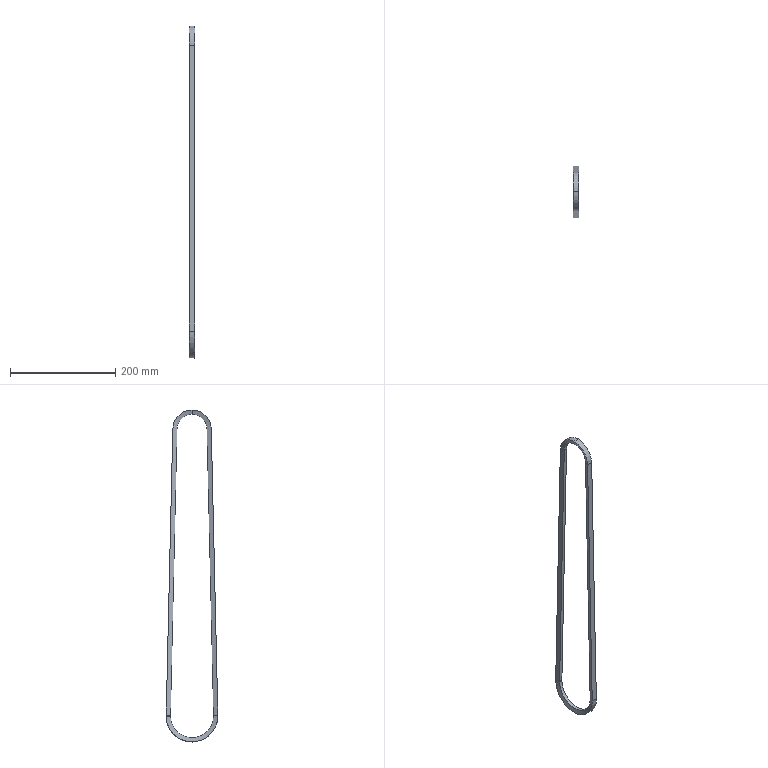Part | STEP file | Long V-belt | 1 solid | 24 faces | box 11 x 98 x 629.5 mm | volume 91301 mm3 | cone 8 | cylinder 8 | plane 8 | commonest cylinder face diameters 57 x2 73 x2 82 x2 98 x2
STEP:
#1=CARTESIAN_POINT('',(3.054,41.,0.));
#2=VERTEX_POINT('',#1);
#3=CARTESIAN_POINT('',(3.054,0.,-41.));
#4=VERTEX_POINT('',#3);
#5=CARTESIAN_POINT('',(3.054,0.,0.));
#6=DIRECTION('',(-1.,0.,0.));
#7=DIRECTION('',(0.,1.,0.));
#8=AXIS2_PLACEMENT_3D('',#5,#6,#7);
#9=CIRCLE('',#8,41.);
#10=EDGE_CURVE('',#2,#4,#9,.T.);
#11=ORIENTED_EDGE('',*,*,#10,.T.);
#12=CARTESIAN_POINT('',(5.5,0.,-49.));
#13=VERTEX_POINT('',#12);
#14=CARTESIAN_POINT('',(3.054,0.,-41.));
#15=DIRECTION('',(0.2924,0.,-0.9563));
#16=VECTOR('',#15,1000.);
#17=LINE('',#14,#16);
#18=EDGE_CURVE('',#4,#13,#17,.T.);
#19=ORIENTED_EDGE('',*,*,#18,.T.);
#20=CARTESIAN_POINT('',(5.5,49.,0.));
#21=VERTEX_POINT('',#20);
#22=CARTESIAN_POINT('',(5.5,0.,0.));
#23=DIRECTION('',(-1.,0.,0.));
#24=DIRECTION('',(0.,1.,0.));
#25=AXIS2_PLACEMENT_3D('',#22,#23,#24);
#26=CIRCLE('',#25,49.);
#27=EDGE_CURVE('',#21,#13,#26,.T.);
#28=ORIENTED_EDGE('',*,*,#27,.F.);
#29=CARTESIAN_POINT('',(3.054,41.,0.));
#30=DIRECTION('',(0.2924,0.9563,0.));
#31=VECTOR('',#30,1000.);
#32=LINE('',#29,#31);
#33=EDGE_CURVE('',#2,#21,#32,.T.);
#34=ORIENTED_EDGE('',*,*,#33,.F.);
#35=EDGE_LOOP('',(#11,#19,#28,#34));
#36=FACE_OUTER_BOUND('',#35,.T.);
#37=CARTESIAN_POINT('',(3.054,0.,0.));
#38=DIRECTION('',(1.,0.,0.));
#39=DIRECTION('',(0.,0.,-1.));
#40=AXIS2_PLACEMENT_3D('',#37,#38,#39);
#41=CONICAL_SURFACE('',#40,41.,1.274);
#42=ADVANCED_FACE('',(#36),#41,.F.);
#43=CARTESIAN_POINT('',(5.5,-36.5,544.098));
#44=VERTEX_POINT('',#43);
#45=CARTESIAN_POINT('',(5.5,0.,580.5));
#46=VERTEX_POINT('',#45);
#47=CARTESIAN_POINT('',(5.5,0.,544.));
#48=DIRECTION('',(-1.,0.,0.));
#49=DIRECTION('',(0.,-1.,0.));
#50=AXIS2_PLACEMENT_3D('',#47,#48,#49);
#51=CIRCLE('',#50,36.5);
#52=EDGE_CURVE('',#44,#46,#51,.T.);
#53=ORIENTED_EDGE('',*,*,#52,.T.);
#54=CARTESIAN_POINT('',(-5.5,0.,580.5));
#55=VERTEX_POINT('',#54);
#56=CARTESIAN_POINT('',(0.,0.,580.5));
#57=DIRECTION('',(-1.,0.,0.));
#58=VECTOR('',#57,1000.);
#59=LINE('',#56,#58);
#60=EDGE_CURVE('',#46,#55,#59,.T.);
#61=ORIENTED_EDGE('',*,*,#60,.T.);
#62=CARTESIAN_POINT('',(-5.5,-36.5,544.098));
#63=VERTEX_POINT('',#62);
#64=CARTESIAN_POINT('',(-5.5,0.,544.));
#65=DIRECTION('',(-1.,0.,0.));
#66=DIRECTION('',(0.,-1.,0.));
#67=AXIS2_PLACEMENT_3D('',#64,#65,#66);
#68=CIRCLE('',#67,36.5);
#69=EDGE_CURVE('',#63,#55,#68,.T.);
#70=ORIENTED_EDGE('',*,*,#69,.F.);
#71=CARTESIAN_POINT('',(0.,-36.5,544.098));
#72=DIRECTION('',(1.,0.,0.));
#73=VECTOR('',#72,1000.);
#74=LINE('',#71,#73);
#75=EDGE_CURVE('',#63,#44,#74,.T.);
#76=ORIENTED_EDGE('',*,*,#75,.T.);
#77=EDGE_LOOP('',(#53,#61,#70,#76));
#78=FACE_OUTER_BOUND('',#77,.T.);
#79=CARTESIAN_POINT('',(0.,0.,544.));
#80=DIRECTION('',(-1.,0.,0.));
#81=DIRECTION('',(0.,0.,1.));
#82=AXIS2_PLACEMENT_3D('',#79,#80,#81);
#83=CYLINDRICAL_SURFACE('',#82,36.5);
#84=ADVANCED_FACE('',(#78),#83,.T.);
#85=CARTESIAN_POINT('',(3.054,0.,572.5));
#86=VERTEX_POINT('',#85);
#87=CARTESIAN_POINT('',(3.054,28.5,544.));
#88=VERTEX_POINT('',#87);
#89=CARTESIAN_POINT('',(3.054,0.,544.));
#90=DIRECTION('',(-1.,0.,0.));
#91=DIRECTION('',(0.,-1.,0.));
#92=AXIS2_PLACEMENT_3D('',#89,#90,#91);
#93=CIRCLE('',#92,28.5);
#94=EDGE_CURVE('',#86,#88,#93,.T.);
#95=ORIENTED_EDGE('',*,*,#94,.F.);
#96=CARTESIAN_POINT('',(-3.054,0.,572.5));
#97=VERTEX_POINT('',#96);
#98=CARTESIAN_POINT('',(0.,0.,572.5));
#99=DIRECTION('',(-1.,0.,0.));
#100=VECTOR('',#99,1000.);
#101=LINE('',#98,#100);
#102=EDGE_CURVE('',#86,#97,#101,.T.);
#103=ORIENTED_EDGE('',*,*,#102,.T.);
#104=CARTESIAN_POINT('',(-3.054,28.5,544.));
#105=VERTEX_POINT('',#104);
#106=CARTESIAN_POINT('',(-3.054,0.,544.));
#107=DIRECTION('',(-1.,0.,0.));
#108=DIRECTION('',(0.,-1.,0.));
#109=AXIS2_PLACEMENT_3D('',#106,#107,#108);
#110=CIRCLE('',#109,28.5);
#111=EDGE_CURVE('',#97,#105,#110,.T.);
#112=ORIENTED_EDGE('',*,*,#111,.T.);
#113=CARTESIAN_POINT('',(-3.054,28.5,544.));
#114=DIRECTION('',(1.,0.,0.));
#115=VECTOR('',#114,1000.);
#116=LINE('',#113,#115);
#117=EDGE_CURVE('',#105,#88,#116,.T.);
#118=ORIENTED_EDGE('',*,*,#117,.T.);
#119=EDGE_LOOP('',(#95,#103,#112,#118));
#120=FACE_OUTER_BOUND('',#119,.T.);
#121=CARTESIAN_POINT('',(0.,0.,544.));
#122=DIRECTION('',(-1.,0.,0.));
#123=DIRECTION('',(0.,0.,1.));
#124=AXIS2_PLACEMENT_3D('',#121,#122,#123);
#125=CYLINDRICAL_SURFACE('',#124,28.5);
#126=ADVANCED_FACE('',(#120),#125,.F.);
#127=ORIENTED_EDGE('',*,*,#111,.F.);
#128=CARTESIAN_POINT('',(-5.5,0.,580.5));
#129=DIRECTION('',(-0.2924,0.,0.9563));
#130=VECTOR('',#129,1000.);
#131=LINE('',#128,#130);
#132=EDGE_CURVE('',#97,#55,#131,.T.);
#133=ORIENTED_EDGE('',*,*,#132,.T.);
#134=CARTESIAN_POINT('',(-5.5,36.5,544.098));
#135=VERTEX_POINT('',#134);
#136=CARTESIAN_POINT('',(-5.5,0.,544.));
#137=DIRECTION('',(-1.,0.,0.));
#138=DIRECTION('',(0.,-1.,0.));
#139=AXIS2_PLACEMENT_3D('',#136,#137,#138);
#140=CIRCLE('',#139,36.5);
#141=EDGE_CURVE('',#55,#135,#140,.T.);
#142=ORIENTED_EDGE('',*,*,#141,.T.);
#143=CARTESIAN_POINT('',(-5.5,36.5,544.098));
#144=CARTESIAN_POINT('',(-4.685,33.833,544.063));
#145=CARTESIAN_POINT('',(-3.869,31.167,544.031));
#146=CARTESIAN_POINT('',(-3.054,28.5,544.));
#147=B_SPLINE_CURVE_WITH_KNOTS('',3,(#143,#144,#145,#146),.UNSPECIFIED.,.F.,.F.,(4,4),(0.000000346,0.008366),.UNSPECIFIED.);
#148=EDGE_CURVE('',#135,#105,#147,.T.);
#149=ORIENTED_EDGE('',*,*,#148,.T.);
#150=EDGE_LOOP('',(#127,#133,#142,#149));
#151=FACE_OUTER_BOUND('',#150,.T.);
#152=CARTESIAN_POINT('',(-5.5,0.,544.));
#153=DIRECTION('',(-1.,0.,0.));
#154=DIRECTION('',(0.,0.,1.));
#155=AXIS2_PLACEMENT_3D('',#152,#153,#154);
#156=CONICAL_SURFACE('',#155,36.5,1.274);
#157=ADVANCED_FACE('',(#151),#156,.F.);
#158=CARTESIAN_POINT('',(-5.5,-48.953,2.155));
#159=VERTEX_POINT('',#158);
#160=CARTESIAN_POINT('',(5.5,-48.953,2.155));
#161=VERTEX_POINT('',#160);
#162=CARTESIAN_POINT('',(0.,-48.953,2.155));
#163=DIRECTION('',(1.,0.,0.));
#164=VECTOR('',#163,1000.);
#165=LINE('',#162,#164);
#166=EDGE_CURVE('',#159,#161,#165,.T.);
#167=ORIENTED_EDGE('',*,*,#166,.T.);
#168=CARTESIAN_POINT('',(5.5,-48.955,2.067));
#169=DIRECTION('',(0.,0.02297,0.9997));
#170=VECTOR('',#169,1000.);
#171=LINE('',#168,#170);
#172=EDGE_CURVE('',#161,#44,#171,.T.);
#173=ORIENTED_EDGE('',*,*,#172,.T.);
#174=ORIENTED_EDGE('',*,*,#75,.F.);
#175=CARTESIAN_POINT('',(-5.5,-48.955,2.067));
#176=DIRECTION('',(0.,0.02297,0.9997));
#177=VECTOR('',#176,1000.);
#178=LINE('',#175,#177);
#179=EDGE_CURVE('',#159,#63,#178,.T.);
#180=ORIENTED_EDGE('',*,*,#179,.F.);
#181=EDGE_LOOP('',(#167,#173,#174,#180));
#182=FACE_OUTER_BOUND('',#181,.T.);
#183=CARTESIAN_POINT('',(5.5,-48.955,2.067));
#184=DIRECTION('',(0.,0.9997,-0.02297));
#185=DIRECTION('',(0.,0.02297,0.9997));
#186=AXIS2_PLACEMENT_3D('',#183,#184,#185);
#187=PLANE('',#186);
#188=ADVANCED_FACE('',(#182),#187,.F.);
#189=CARTESIAN_POINT('',(-3.054,-28.5,544.));
#190=VERTEX_POINT('',#189);
#191=CARTESIAN_POINT('',(3.054,-28.5,544.));
#192=VERTEX_POINT('',#191);
#193=CARTESIAN_POINT('',(-3.054,-28.5,544.));
#194=DIRECTION('',(1.,0.,0.));
#195=VECTOR('',#194,1000.);
#196=LINE('',#193,#195);
#197=EDGE_CURVE('',#190,#192,#196,.T.);
#198=ORIENTED_EDGE('',*,*,#197,.T.);
#199=CARTESIAN_POINT('',(3.054,-40.957,1.883));
#200=VERTEX_POINT('',#199);
#201=CARTESIAN_POINT('',(3.054,-40.957,1.883));
#202=DIRECTION('',(0.,0.02297,0.9997));
#203=VECTOR('',#202,1000.);
#204=LINE('',#201,#203);
#205=EDGE_CURVE('',#200,#192,#204,.T.);
#206=ORIENTED_EDGE('',*,*,#205,.F.);
#207=CARTESIAN_POINT('',(-3.054,-40.957,1.883));
#208=VERTEX_POINT('',#207);
#209=CARTESIAN_POINT('',(-3.054,-40.957,1.883));
#210=DIRECTION('',(1.,0.,0.));
#211=VECTOR('',#210,1000.);
#212=LINE('',#209,#211);
#213=EDGE_CURVE('',#208,#200,#212,.T.);
#214=ORIENTED_EDGE('',*,*,#213,.F.);
#215=CARTESIAN_POINT('',(-3.054,-40.957,1.883));
#216=DIRECTION('',(0.,0.02297,0.9997));
#217=VECTOR('',#216,1000.);
#218=LINE('',#215,#217);
#219=EDGE_CURVE('',#208,#190,#218,.T.);
#220=ORIENTED_EDGE('',*,*,#219,.T.);
#221=EDGE_LOOP('',(#198,#206,#214,#220));
#222=FACE_OUTER_BOUND('',#221,.T.);
#223=CARTESIAN_POINT('',(-3.054,-40.957,1.883));
#224=DIRECTION('',(0.,-0.9997,0.02297));
#225=DIRECTION('',(0.,-0.02297,-0.9997));
#226=AXIS2_PLACEMENT_3D('',#223,#224,#225);
#227=PLANE('',#226);
#228=ADVANCED_FACE('',(#222),#227,.F.);
#229=ORIENTED_EDGE('',*,*,#179,.T.);
#230=CARTESIAN_POINT('',(-5.5,-36.5,544.098));
#231=CARTESIAN_POINT('',(-4.685,-33.833,544.063));
#232=CARTESIAN_POINT('',(-3.869,-31.167,544.031));
#233=CARTESIAN_POINT('',(-3.054,-28.5,544.));
#234=B_SPLINE_CURVE_WITH_KNOTS('',3,(#230,#231,#232,#233),.UNSPECIFIED.,.F.,.F.,(4,4),(0.000000346,0.008366),.UNSPECIFIED.);
#235=EDGE_CURVE('',#63,#190,#234,.T.);
#236=ORIENTED_EDGE('',*,*,#235,.T.);
#237=ORIENTED_EDGE('',*,*,#219,.F.);
#238=CARTESIAN_POINT('',(-5.5,-48.953,2.155));
#239=CARTESIAN_POINT('',(-4.685,-46.287,2.065));
#240=CARTESIAN_POINT('',(-3.869,-43.622,1.975));
#241=CARTESIAN_POINT('',(-3.054,-40.957,1.883));
#242=B_SPLINE_CURVE_WITH_KNOTS('',3,(#238,#239,#240,#241),.UNSPECIFIED.,.F.,.F.,(4,4),(0.000000684,0.008367),.UNSPECIFIED.);
#243=EDGE_CURVE('',#159,#208,#242,.T.);
#244=ORIENTED_EDGE('',*,*,#243,.F.);
#245=EDGE_LOOP('',(#229,#236,#237,#244));
#246=FACE_OUTER_BOUND('',#245,.T.);
#247=CARTESIAN_POINT('',(-3.054,-40.957,1.883));
#248=DIRECTION('',(0.9563,-0.2923,0.006716));
#249=DIRECTION('',(0.2923,0.9563,0.));
#250=AXIS2_PLACEMENT_3D('',#247,#248,#249);
#251=PLANE('',#250);
#252=ADVANCED_FACE('',(#246),#251,.F.);
#253=ORIENTED_EDGE('',*,*,#205,.T.);
#254=CARTESIAN_POINT('',(3.054,-28.5,544.));
#255=CARTESIAN_POINT('',(3.869,-31.167,544.031));
#256=CARTESIAN_POINT('',(4.685,-33.833,544.063));
#257=CARTESIAN_POINT('',(5.5,-36.5,544.098));
#258=B_SPLINE_CURVE_WITH_KNOTS('',3,(#254,#255,#256,#257),.UNSPECIFIED.,.F.,.F.,(4,4),(0.000000209,0.008366),.UNSPECIFIED.);
#259=EDGE_CURVE('',#192,#44,#258,.T.);
#260=ORIENTED_EDGE('',*,*,#259,.T.);
#261=ORIENTED_EDGE('',*,*,#172,.F.);
#262=CARTESIAN_POINT('',(3.054,-40.957,1.883));
#263=CARTESIAN_POINT('',(3.869,-43.622,1.975));
#264=CARTESIAN_POINT('',(4.685,-46.287,2.065));
#265=CARTESIAN_POINT('',(5.5,-48.953,2.155));
#266=B_SPLINE_CURVE_WITH_KNOTS('',3,(#262,#263,#264,#265),.UNSPECIFIED.,.F.,.F.,(4,4),(0.000000684,0.008367),.UNSPECIFIED.);
#267=EDGE_CURVE('',#200,#161,#266,.T.);
#268=ORIENTED_EDGE('',*,*,#267,.F.);
#269=EDGE_LOOP('',(#253,#260,#261,#268));
#270=FACE_OUTER_BOUND('',#269,.T.);
#271=CARTESIAN_POINT('',(3.054,-40.957,1.883));
#272=DIRECTION('',(-0.9563,-0.2923,0.006716));
#273=DIRECTION('',(0.2923,-0.9563,0.));
#274=AXIS2_PLACEMENT_3D('',#271,#272,#273);
#275=PLANE('',#274);
#276=ADVANCED_FACE('',(#270),#275,.F.);
#277=CARTESIAN_POINT('',(-5.5,49.,0.));
#278=VERTEX_POINT('',#277);
#279=CARTESIAN_POINT('',(-5.5,0.,0.));
#280=DIRECTION('',(-1.,0.,0.));
#281=DIRECTION('',(0.,1.,0.));
#282=AXIS2_PLACEMENT_3D('',#279,#280,#281);
#283=CIRCLE('',#282,49.);
#284=EDGE_CURVE('',#278,#159,#283,.T.);
#285=ORIENTED_EDGE('',*,*,#284,.F.);
#286=CARTESIAN_POINT('',(5.5,49.,0.));
#287=DIRECTION('',(-1.,0.,0.));
#288=VECTOR('',#287,1000.);
#289=LINE('',#286,#288);
#290=EDGE_CURVE('',#21,#278,#289,.T.);
#291=ORIENTED_EDGE('',*,*,#290,.F.);
#292=ORIENTED_EDGE('',*,*,#27,.T.);
#293=CARTESIAN_POINT('',(5.5,0.,0.));
#294=DIRECTION('',(-1.,0.,0.));
#295=DIRECTION('',(0.,1.,0.));
#296=AXIS2_PLACEMENT_3D('',#293,#294,#295);
#297=CIRCLE('',#296,49.);
#298=EDGE_CURVE('',#13,#161,#297,.T.);
#299=ORIENTED_EDGE('',*,*,#298,.T.);
#300=ORIENTED_EDGE('',*,*,#166,.F.);
#301=EDGE_LOOP('',(#285,#291,#292,#299,#300));
#302=FACE_OUTER_BOUND('',#301,.T.);
#303=CARTESIAN_POINT('',(0.,0.,0.));
#304=DIRECTION('',(-1.,0.,0.));
#305=DIRECTION('',(0.,0.,1.));
#306=AXIS2_PLACEMENT_3D('',#303,#304,#305);
#307=CYLINDRICAL_SURFACE('',#306,49.);
#308=ADVANCED_FACE('',(#302),#307,.T.);
#309=CARTESIAN_POINT('',(-5.5,48.953,2.155));
#310=VERTEX_POINT('',#309);
#311=CARTESIAN_POINT('',(5.5,48.953,2.155));
#312=VERTEX_POINT('',#311);
#313=CARTESIAN_POINT('',(0.,48.953,2.155));
#314=DIRECTION('',(1.,0.,0.));
#315=VECTOR('',#314,1000.);
#316=LINE('',#313,#315);
#317=EDGE_CURVE('',#310,#312,#316,.T.);
#318=ORIENTED_EDGE('',*,*,#317,.T.);
#319=CARTESIAN_POINT('',(5.5,0.,0.));
#320=DIRECTION('',(-1.,0.,0.));
#321=DIRECTION('',(0.,0.9989,0.04593));
#322=AXIS2_PLACEMENT_3D('',#319,#320,#321);
#323=CIRCLE('',#322,49.);
#324=EDGE_CURVE('',#312,#21,#323,.T.);
#325=ORIENTED_EDGE('',*,*,#324,.T.);
#326=ORIENTED_EDGE('',*,*,#290,.T.);
#327=CARTESIAN_POINT('',(-5.5,0.,0.));
#328=DIRECTION('',(-1.,0.,0.));
#329=DIRECTION('',(0.,0.9989,0.04593));
#330=AXIS2_PLACEMENT_3D('',#327,#328,#329);
#331=CIRCLE('',#330,49.);
#332=EDGE_CURVE('',#310,#278,#331,.T.);
#333=ORIENTED_EDGE('',*,*,#332,.F.);
#334=EDGE_LOOP('',(#318,#325,#326,#333));
#335=FACE_OUTER_BOUND('',#334,.T.);
#336=CARTESIAN_POINT('',(0.,0.,0.));
#337=DIRECTION('',(-1.,0.,0.));
#338=DIRECTION('',(0.,0.,1.));
#339=AXIS2_PLACEMENT_3D('',#336,#337,#338);
#340=CYLINDRICAL_SURFACE('',#339,49.);
#341=ADVANCED_FACE('',(#335),#340,.T.);
#342=ORIENTED_EDGE('',*,*,#213,.T.);
#343=CARTESIAN_POINT('',(3.054,0.,0.));
#344=DIRECTION('',(-1.,0.,0.));
#345=DIRECTION('',(0.,1.,0.));
#346=AXIS2_PLACEMENT_3D('',#343,#344,#345);
#347=CIRCLE('',#346,41.);
#348=EDGE_CURVE('',#4,#200,#347,.T.);
#349=ORIENTED_EDGE('',*,*,#348,.F.);
#350=ORIENTED_EDGE('',*,*,#10,.F.);
#351=CARTESIAN_POINT('',(-3.054,41.,0.));
#352=VERTEX_POINT('',#351);
#353=CARTESIAN_POINT('',(-3.054,41.,0.));
#354=DIRECTION('',(1.,0.,0.));
#355=VECTOR('',#354,1000.);
#356=LINE('',#353,#355);
#357=EDGE_CURVE('',#352,#2,#356,.T.);
#358=ORIENTED_EDGE('',*,*,#357,.F.);
#359=CARTESIAN_POINT('',(-3.054,0.,0.));
#360=DIRECTION('',(-1.,0.,0.));
#361=DIRECTION('',(0.,1.,0.));
#362=AXIS2_PLACEMENT_3D('',#359,#360,#361);
#363=CIRCLE('',#362,41.);
#364=EDGE_CURVE('',#352,#208,#363,.T.);
#365=ORIENTED_EDGE('',*,*,#364,.T.);
#366=EDGE_LOOP('',(#342,#349,#350,#358,#365));
#367=FACE_OUTER_BOUND('',#366,.T.);
#368=CARTESIAN_POINT('',(0.,0.,0.));
#369=DIRECTION('',(-1.,0.,0.));
#370=DIRECTION('',(0.,0.,1.));
#371=AXIS2_PLACEMENT_3D('',#368,#369,#370);
#372=CYLINDRICAL_SURFACE('',#371,41.);
#373=ADVANCED_FACE('',(#367),#372,.F.);
#374=ORIENTED_EDGE('',*,*,#243,.T.);
#375=ORIENTED_EDGE('',*,*,#364,.F.);
#376=CARTESIAN_POINT('',(-3.054,41.,0.));
#377=DIRECTION('',(0.2924,-0.9563,0.));
#378=VECTOR('',#377,1000.);
#379=LINE('',#376,#378);
#380=EDGE_CURVE('',#278,#352,#379,.T.);
#381=ORIENTED_EDGE('',*,*,#380,.F.);
#382=ORIENTED_EDGE('',*,*,#284,.T.);
#383=EDGE_LOOP('',(#374,#375,#381,#382));
#384=FACE_OUTER_BOUND('',#383,.T.);
#385=CARTESIAN_POINT('',(-5.5,0.,0.));
#386=DIRECTION('',(-1.,0.,0.));
#387=DIRECTION('',(0.,0.,1.));
#388=AXIS2_PLACEMENT_3D('',#385,#386,#387);
#389=CONICAL_SURFACE('',#388,49.,1.274);
#390=ADVANCED_FACE('',(#384),#389,.F.);
#391=ORIENTED_EDGE('',*,*,#18,.F.);
#392=ORIENTED_EDGE('',*,*,#348,.T.);
#393=ORIENTED_EDGE('',*,*,#267,.T.);
#394=ORIENTED_EDGE('',*,*,#298,.F.);
#395=EDGE_LOOP('',(#391,#392,#393,#394));
#396=FACE_OUTER_BOUND('',#395,.T.);
#397=CARTESIAN_POINT('',(3.054,0.,0.));
#398=DIRECTION('',(1.,0.,0.));
#399=DIRECTION('',(0.,0.,-1.));
#400=AXIS2_PLACEMENT_3D('',#397,#398,#399);
#401=CONICAL_SURFACE('',#400,41.,1.274);
#402=ADVANCED_FACE('',(#396),#401,.F.);
#403=ORIENTED_EDGE('',*,*,#357,.T.);
#404=CARTESIAN_POINT('',(3.054,40.957,1.883));
#405=VERTEX_POINT('',#404);
#406=CARTESIAN_POINT('',(3.054,0.,0.));
#407=DIRECTION('',(-1.,0.,0.));
#408=DIRECTION('',(0.,0.9989,0.04593));
#409=AXIS2_PLACEMENT_3D('',#406,#407,#408);
#410=CIRCLE('',#409,41.);
#411=EDGE_CURVE('',#405,#2,#410,.T.);
#412=ORIENTED_EDGE('',*,*,#411,.F.);
#413=CARTESIAN_POINT('',(-3.054,40.957,1.883));
#414=VERTEX_POINT('',#413);
#415=CARTESIAN_POINT('',(-3.054,40.957,1.883));
#416=DIRECTION('',(1.,0.,0.));
#417=VECTOR('',#416,1000.);
#418=LINE('',#415,#417);
#419=EDGE_CURVE('',#414,#405,#418,.T.);
#420=ORIENTED_EDGE('',*,*,#419,.F.);
#421=CARTESIAN_POINT('',(-3.054,0.,0.));
#422=DIRECTION('',(-1.,0.,0.));
#423=DIRECTION('',(0.,0.9989,0.04593));
#424=AXIS2_PLACEMENT_3D('',#421,#422,#423);
#425=CIRCLE('',#424,41.);
#426=EDGE_CURVE('',#414,#352,#425,.T.);
#427=ORIENTED_EDGE('',*,*,#426,.T.);
#428=EDGE_LOOP('',(#403,#412,#420,#427));
#429=FACE_OUTER_BOUND('',#428,.T.);
#430=CARTESIAN_POINT('',(0.,0.,0.));
#431=DIRECTION('',(-1.,0.,0.));
#432=DIRECTION('',(0.,0.,1.));
#433=AXIS2_PLACEMENT_3D('',#430,#431,#432);
#434=CYLINDRICAL_SURFACE('',#433,41.);
#435=ADVANCED_FACE('',(#429),#434,.F.);
#436=ORIENTED_EDGE('',*,*,#332,.T.);
#437=ORIENTED_EDGE('',*,*,#380,.T.);
#438=ORIENTED_EDGE('',*,*,#426,.F.);
#439=CARTESIAN_POINT('',(-5.5,48.953,2.155));
#440=CARTESIAN_POINT('',(-4.685,46.287,2.065));
#441=CARTESIAN_POINT('',(-3.869,43.622,1.975));
#442=CARTESIAN_POINT('',(-3.054,40.957,1.883));
#443=B_SPLINE_CURVE_WITH_KNOTS('',3,(#439,#440,#441,#442),.UNSPECIFIED.,.F.,.F.,(4,4),(0.000000684,0.008367),.UNSPECIFIED.);
#444=EDGE_CURVE('',#310,#414,#443,.T.);
#445=ORIENTED_EDGE('',*,*,#444,.F.);
#446=EDGE_LOOP('',(#436,#437,#438,#445));
#447=FACE_OUTER_BOUND('',#446,.T.);
#448=CARTESIAN_POINT('',(-5.5,0.,0.));
#449=DIRECTION('',(-1.,0.,0.));
#450=DIRECTION('',(0.,0.,1.));
#451=AXIS2_PLACEMENT_3D('',#448,#449,#450);
#452=CONICAL_SURFACE('',#451,49.,1.274);
#453=ADVANCED_FACE('',(#447),#452,.F.);
#454=ORIENTED_EDGE('',*,*,#411,.T.);
#455=ORIENTED_EDGE('',*,*,#33,.T.);
#456=ORIENTED_EDGE('',*,*,#324,.F.);
#457=CARTESIAN_POINT('',(3.054,40.957,1.883));
#458=CARTESIAN_POINT('',(3.869,43.622,1.975));
#459=CARTESIAN_POINT('',(4.685,46.287,2.065));
#460=CARTESIAN_POINT('',(5.5,48.953,2.155));
#461=B_SPLINE_CURVE_WITH_KNOTS('',3,(#457,#458,#459,#460),.UNSPECIFIED.,.F.,.F.,(4,4),(0.000000209,0.008366),.UNSPECIFIED.);
#462=EDGE_CURVE('',#405,#312,#461,.T.);
#463=ORIENTED_EDGE('',*,*,#462,.F.);
#464=EDGE_LOOP('',(#454,#455,#456,#463));
#465=FACE_OUTER_BOUND('',#464,.T.);
#466=CARTESIAN_POINT('',(3.054,0.,0.));
#467=DIRECTION('',(1.,0.,0.));
#468=DIRECTION('',(0.,0.,-1.));
#469=AXIS2_PLACEMENT_3D('',#466,#467,#468);
#470=CONICAL_SURFACE('',#469,41.,1.274);
#471=ADVANCED_FACE('',(#465),#470,.F.);
#472=ORIENTED_EDGE('',*,*,#60,.F.);
#473=CARTESIAN_POINT('',(5.5,36.5,544.098));
#474=VERTEX_POINT('',#473);
#475=CARTESIAN_POINT('',(5.5,0.,544.));
#476=DIRECTION('',(-1.,0.,0.));
#477=DIRECTION('',(0.,-1.,0.));
#478=AXIS2_PLACEMENT_3D('',#475,#476,#477);
#479=CIRCLE('',#478,36.5);
#480=EDGE_CURVE('',#46,#474,#479,.T.);
#481=ORIENTED_EDGE('',*,*,#480,.T.);
#482=CARTESIAN_POINT('',(0.,36.5,544.098));
#483=DIRECTION('',(1.,0.,0.));
#484=VECTOR('',#483,1000.);
#485=LINE('',#482,#484);
#486=EDGE_CURVE('',#135,#474,#485,.T.);
#487=ORIENTED_EDGE('',*,*,#486,.F.);
#488=ORIENTED_EDGE('',*,*,#141,.F.);
#489=EDGE_LOOP('',(#472,#481,#487,#488));
#490=FACE_OUTER_BOUND('',#489,.T.);
#491=CARTESIAN_POINT('',(0.,0.,544.));
#492=DIRECTION('',(-1.,0.,0.));
#493=DIRECTION('',(0.,0.,1.));
#494=AXIS2_PLACEMENT_3D('',#491,#492,#493);
#495=CYLINDRICAL_SURFACE('',#494,36.5);
#496=ADVANCED_FACE('',(#490),#495,.T.);
#497=ORIENTED_EDGE('',*,*,#102,.F.);
#498=CARTESIAN_POINT('',(3.054,0.,544.));
#499=DIRECTION('',(-1.,0.,0.));
#500=DIRECTION('',(0.,-1.,0.));
#501=AXIS2_PLACEMENT_3D('',#498,#499,#500);
#502=CIRCLE('',#501,28.5);
#503=EDGE_CURVE('',#192,#86,#502,.T.);
#504=ORIENTED_EDGE('',*,*,#503,.F.);
#505=ORIENTED_EDGE('',*,*,#197,.F.);
#506=CARTESIAN_POINT('',(-3.054,0.,544.));
#507=DIRECTION('',(-1.,0.,0.));
#508=DIRECTION('',(0.,-1.,0.));
#509=AXIS2_PLACEMENT_3D('',#506,#507,#508);
#510=CIRCLE('',#509,28.5);
#511=EDGE_CURVE('',#190,#97,#510,.T.);
#512=ORIENTED_EDGE('',*,*,#511,.T.);
#513=EDGE_LOOP('',(#497,#504,#505,#512));
#514=FACE_OUTER_BOUND('',#513,.T.);
#515=CARTESIAN_POINT('',(0.,0.,544.));
#516=DIRECTION('',(-1.,0.,0.));
#517=DIRECTION('',(0.,0.,1.));
#518=AXIS2_PLACEMENT_3D('',#515,#516,#517);
#519=CYLINDRICAL_SURFACE('',#518,28.5);
#520=ADVANCED_FACE('',(#514),#519,.F.);
#521=ORIENTED_EDGE('',*,*,#132,.F.);
#522=ORIENTED_EDGE('',*,*,#511,.F.);
#523=ORIENTED_EDGE('',*,*,#235,.F.);
#524=ORIENTED_EDGE('',*,*,#69,.T.);
#525=EDGE_LOOP('',(#521,#522,#523,#524));
#526=FACE_OUTER_BOUND('',#525,.T.);
#527=CARTESIAN_POINT('',(-5.5,0.,544.));
#528=DIRECTION('',(-1.,0.,0.));
#529=DIRECTION('',(0.,0.,1.));
#530=AXIS2_PLACEMENT_3D('',#527,#528,#529);
#531=CONICAL_SURFACE('',#530,36.5,1.274);
#532=ADVANCED_FACE('',(#526),#531,.F.);
#533=CARTESIAN_POINT('',(3.054,28.5,544.));
#534=CARTESIAN_POINT('',(3.869,31.167,544.031));
#535=CARTESIAN_POINT('',(4.685,33.833,544.063));
#536=CARTESIAN_POINT('',(5.5,36.5,544.098));
#537=B_SPLINE_CURVE_WITH_KNOTS('',3,(#533,#534,#535,#536),.UNSPECIFIED.,.F.,.F.,(4,4),(0.000000209,0.008366),.UNSPECIFIED.);
#538=EDGE_CURVE('',#88,#474,#537,.T.);
#539=ORIENTED_EDGE('',*,*,#538,.T.);
#540=ORIENTED_EDGE('',*,*,#480,.F.);
#541=ORIENTED_EDGE('',*,*,#52,.F.);
#542=ORIENTED_EDGE('',*,*,#259,.F.);
#543=ORIENTED_EDGE('',*,*,#503,.T.);
#544=ORIENTED_EDGE('',*,*,#94,.T.);
#545=EDGE_LOOP('',(#539,#540,#541,#542,#543,#544));
#546=FACE_OUTER_BOUND('',#545,.T.);
#547=CARTESIAN_POINT('',(3.054,0.,544.));
#548=DIRECTION('',(1.,0.,0.));
#549=DIRECTION('',(0.,0.,-1.));
#550=AXIS2_PLACEMENT_3D('',#547,#548,#549);
#551=CONICAL_SURFACE('',#550,28.5,1.274);
#552=ADVANCED_FACE('',(#546),#551,.F.);
#553=CARTESIAN_POINT('',(-5.5,36.498,544.184));
#554=DIRECTION('',(0.,0.02297,-0.9997));
#555=VECTOR('',#554,1000.);
#556=LINE('',#553,#555);
#557=EDGE_CURVE('',#135,#310,#556,.T.);
#558=ORIENTED_EDGE('',*,*,#557,.F.);
#559=ORIENTED_EDGE('',*,*,#486,.T.);
#560=CARTESIAN_POINT('',(5.5,36.498,544.184));
#561=DIRECTION('',(0.,0.02297,-0.9997));
#562=VECTOR('',#561,1000.);
#563=LINE('',#560,#562);
#564=EDGE_CURVE('',#474,#312,#563,.T.);
#565=ORIENTED_EDGE('',*,*,#564,.T.);
#566=ORIENTED_EDGE('',*,*,#317,.F.);
#567=EDGE_LOOP('',(#558,#559,#565,#566));
#568=FACE_OUTER_BOUND('',#567,.T.);
#569=CARTESIAN_POINT('',(5.5,36.498,544.184));
#570=DIRECTION('',(0.,-0.9997,-0.02297));
#571=DIRECTION('',(0.,0.02297,-0.9997));
#572=AXIS2_PLACEMENT_3D('',#569,#570,#571);
#573=PLANE('',#572);
#574=ADVANCED_FACE('',(#568),#573,.F.);
#575=ORIENTED_EDGE('',*,*,#419,.T.);
#576=CARTESIAN_POINT('',(3.054,28.5,544.));
#577=DIRECTION('',(0.,0.02297,-0.9997));
#578=VECTOR('',#577,1000.);
#579=LINE('',#576,#578);
#580=EDGE_CURVE('',#88,#405,#579,.T.);
#581=ORIENTED_EDGE('',*,*,#580,.F.);
#582=ORIENTED_EDGE('',*,*,#117,.F.);
#583=CARTESIAN_POINT('',(-3.054,28.5,544.));
#584=DIRECTION('',(0.,0.02297,-0.9997));
#585=VECTOR('',#584,1000.);
#586=LINE('',#583,#585);
#587=EDGE_CURVE('',#105,#414,#586,.T.);
#588=ORIENTED_EDGE('',*,*,#587,.T.);
#589=EDGE_LOOP('',(#575,#581,#582,#588));
#590=FACE_OUTER_BOUND('',#589,.T.);
#591=CARTESIAN_POINT('',(-3.054,28.5,544.));
#592=DIRECTION('',(0.,0.9997,0.02297));
#593=DIRECTION('',(0.,-0.02297,0.9997));
#594=AXIS2_PLACEMENT_3D('',#591,#592,#593);
#595=PLANE('',#594);
#596=ADVANCED_FACE('',(#590),#595,.F.);
#597=ORIENTED_EDGE('',*,*,#444,.T.);
#598=ORIENTED_EDGE('',*,*,#587,.F.);
#599=ORIENTED_EDGE('',*,*,#148,.F.);
#600=ORIENTED_EDGE('',*,*,#557,.T.);
#601=EDGE_LOOP('',(#597,#598,#599,#600));
#602=FACE_OUTER_BOUND('',#601,.T.);
#603=CARTESIAN_POINT('',(-3.054,28.5,544.));
#604=DIRECTION('',(0.9563,0.2923,0.006716));
#605=DIRECTION('',(-0.2923,0.9563,0.));
#606=AXIS2_PLACEMENT_3D('',#603,#604,#605);
#607=PLANE('',#606);
#608=ADVANCED_FACE('',(#602),#607,.F.);
#609=ORIENTED_EDGE('',*,*,#462,.T.);
#610=ORIENTED_EDGE('',*,*,#564,.F.);
#611=ORIENTED_EDGE('',*,*,#538,.F.);
#612=ORIENTED_EDGE('',*,*,#580,.T.);
#613=EDGE_LOOP('',(#609,#610,#611,#612));
#614=FACE_OUTER_BOUND('',#613,.T.);
#615=CARTESIAN_POINT('',(3.054,28.5,544.));
#616=DIRECTION('',(-0.9563,0.2923,0.006716));
#617=DIRECTION('',(-0.2923,-0.9563,0.));
#618=AXIS2_PLACEMENT_3D('',#615,#616,#617);
#619=PLANE('',#618);
#620=ADVANCED_FACE('',(#614),#619,.F.);
#621=CLOSED_SHELL('',(#42,#84,#126,#157,#188,#228,#252,#276,#308,#341,#373,#390,#402,#435,#453,#471,#496,#520,#532,#552,#574,#596,#608,#620));
#622=MANIFOLD_SOLID_BREP('',#621);
#623=CARTESIAN_POINT('',(0.,0.,0.));
#624=DIRECTION('',(0.,0.,1.));
#625=DIRECTION('',(1.,0.,0.));
#626=AXIS2_PLACEMENT_3D('',#623,#624,#625);
#627=(LENGTH_UNIT()NAMED_UNIT(*)SI_UNIT(.MILLI.,.METRE.));
#628=UNCERTAINTY_MEASURE_WITH_UNIT(LENGTH_MEASURE(0.00001),#627,'','');
#629=(NAMED_UNIT(*)PLANE_ANGLE_UNIT()SI_UNIT($,.RADIAN.));
#630=(NAMED_UNIT(*)SI_UNIT($,.STERADIAN.)SOLID_ANGLE_UNIT());
#631=(GEOMETRIC_REPRESENTATION_CONTEXT(3)GLOBAL_UNCERTAINTY_ASSIGNED_CONTEXT((#628))GLOBAL_UNIT_ASSIGNED_CONTEXT((#627,#629,#630))REPRESENTATION_CONTEXT('',''));
#632=ADVANCED_BREP_SHAPE_REPRESENTATION('',(#622,#626),#631);